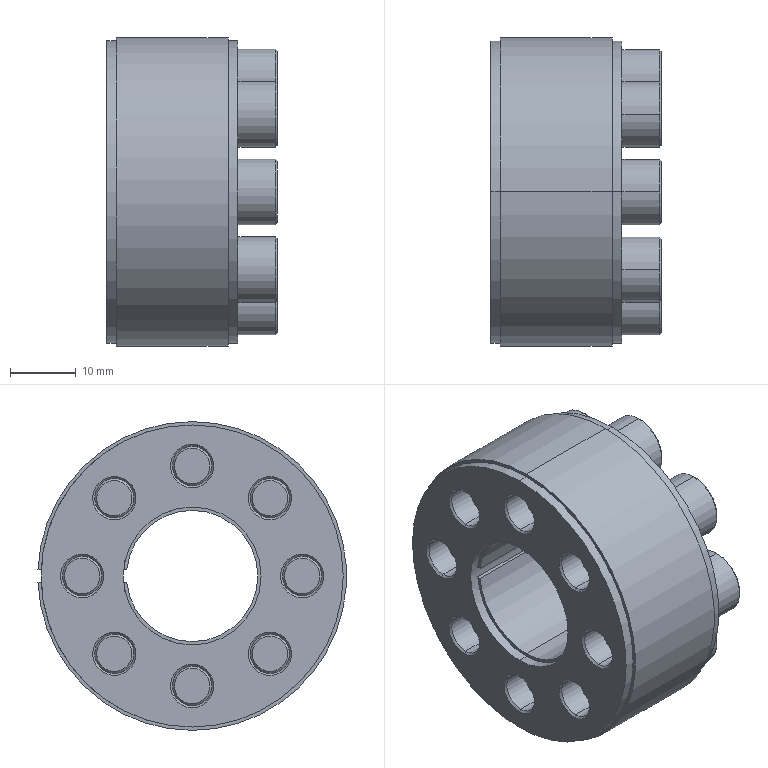Part | SolidWorks | features BaseBody 1 | 1 solid | 174 faces | box 26 x 46.982 x 47 mm | volume 30036 mm3 | plane 82 | cone 48 | cylinder 44 | commonest cylinder face diameters 6 x16 10 x16 20 x3 21 x3 46 x3 47 x3